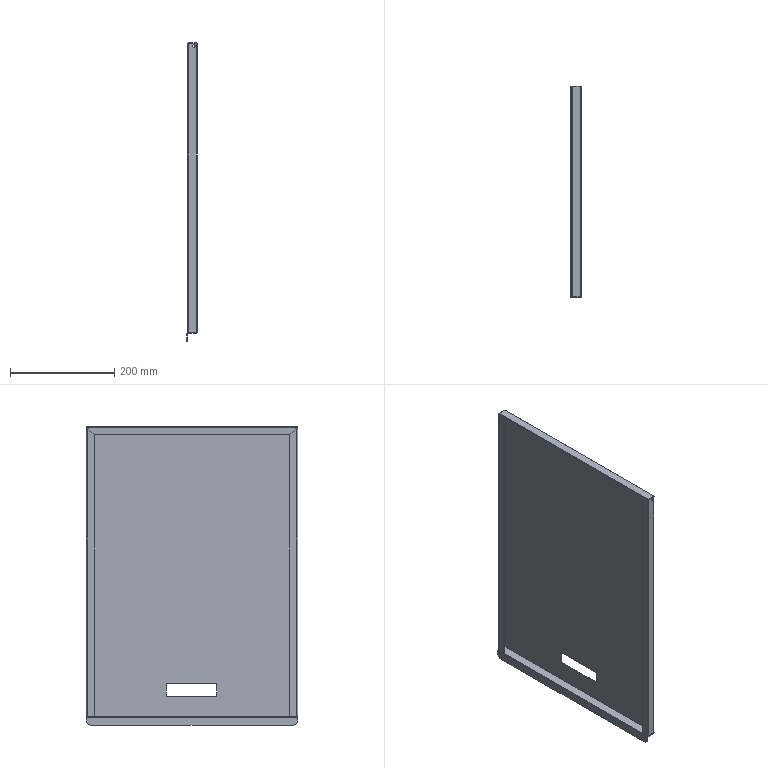Part | 1 solid | 88 faces | box 19.5 x 405 x 572 mm | volume 420245 mm3 | plane 66 | cylinder 22 | commonest cylinder face diameters 0.2 x8 3.2 x8 5.2 x4 20 x2